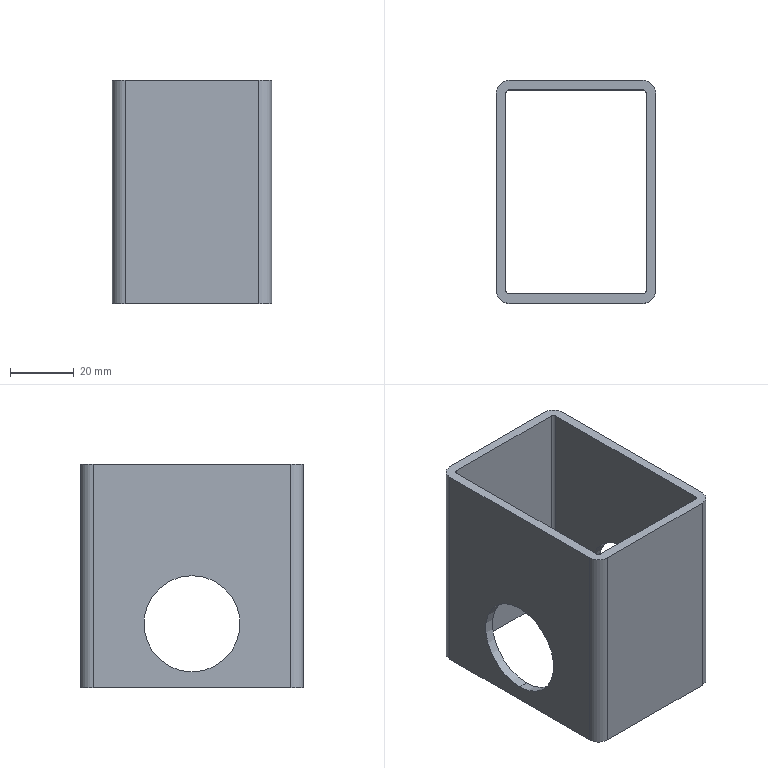Part | SolidWorks | features ExtruThin 1, ICE 1 | 1 solid | 22 faces | box 50 x 70 x 70 mm | volume 42681 mm3 | cylinder 12 | plane 10 | commonest cylinder face diameters 2 x4 8 x4 30.2 x4
STEP:
#1=CARTESIAN_POINT('',(22.,0.,4.9));
#2=VERTEX_POINT('',#1);
#3=CARTESIAN_POINT('',(22.,0.,35.1));
#4=VERTEX_POINT('',#3);
#5=CARTESIAN_POINT('',(22.,0.,20.));
#6=DIRECTION('',(-1.,0.,0.));
#7=DIRECTION('',(0.,0.,1.));
#8=AXIS2_PLACEMENT_3D('',#5,#6,#7);
#9=CIRCLE('',#8,15.1);
#10=EDGE_CURVE('',#2,#4,#9,.T.);
#11=ORIENTED_EDGE('',*,*,#10,.T.);
#12=CARTESIAN_POINT('',(25.,0.,35.1));
#13=VERTEX_POINT('',#12);
#14=CARTESIAN_POINT('',(-25.,0.,35.1));
#15=DIRECTION('',(1.,0.,0.));
#16=VECTOR('',#15,1000.);
#17=LINE('',#14,#16);
#18=EDGE_CURVE('',#4,#13,#17,.T.);
#19=ORIENTED_EDGE('',*,*,#18,.T.);
#20=CARTESIAN_POINT('',(25.,0.,4.9));
#21=VERTEX_POINT('',#20);
#22=CARTESIAN_POINT('',(25.,0.,20.));
#23=DIRECTION('',(1.,0.,0.));
#24=DIRECTION('',(0.,0.,-1.));
#25=AXIS2_PLACEMENT_3D('',#22,#23,#24);
#26=CIRCLE('',#25,15.1);
#27=EDGE_CURVE('',#13,#21,#26,.T.);
#28=ORIENTED_EDGE('',*,*,#27,.T.);
#29=CARTESIAN_POINT('',(-25.,0.,4.9));
#30=DIRECTION('',(1.,0.,0.));
#31=VECTOR('',#30,1000.);
#32=LINE('',#29,#31);
#33=EDGE_CURVE('',#2,#21,#32,.T.);
#34=ORIENTED_EDGE('',*,*,#33,.F.);
#35=EDGE_LOOP('',(#11,#19,#28,#34));
#36=FACE_OUTER_BOUND('',#35,.T.);
#37=CARTESIAN_POINT('',(-25.,0.,20.));
#38=DIRECTION('',(1.,0.,0.));
#39=DIRECTION('',(0.,0.,-1.));
#40=AXIS2_PLACEMENT_3D('',#37,#38,#39);
#41=CYLINDRICAL_SURFACE('',#40,15.1);
#42=ADVANCED_FACE('',(#36),#41,.F.);
#43=CARTESIAN_POINT('',(-25.,0.,35.1));
#44=VERTEX_POINT('',#43);
#45=CARTESIAN_POINT('',(-25.,0.,4.9));
#46=VERTEX_POINT('',#45);
#47=CARTESIAN_POINT('',(-25.,0.,20.));
#48=DIRECTION('',(1.,0.,0.));
#49=DIRECTION('',(0.,0.,-1.));
#50=AXIS2_PLACEMENT_3D('',#47,#48,#49);
#51=CIRCLE('',#50,15.1);
#52=EDGE_CURVE('',#44,#46,#51,.T.);
#53=ORIENTED_EDGE('',*,*,#52,.F.);
#54=CARTESIAN_POINT('',(-22.,0.,35.1));
#55=VERTEX_POINT('',#54);
#56=CARTESIAN_POINT('',(-25.,0.,35.1));
#57=DIRECTION('',(1.,0.,0.));
#58=VECTOR('',#57,1000.);
#59=LINE('',#56,#58);
#60=EDGE_CURVE('',#44,#55,#59,.T.);
#61=ORIENTED_EDGE('',*,*,#60,.T.);
#62=CARTESIAN_POINT('',(-22.,0.,4.9));
#63=VERTEX_POINT('',#62);
#64=CARTESIAN_POINT('',(-22.,0.,20.));
#65=DIRECTION('',(1.,0.,0.));
#66=DIRECTION('',(0.,0.,-1.));
#67=AXIS2_PLACEMENT_3D('',#64,#65,#66);
#68=CIRCLE('',#67,15.1);
#69=EDGE_CURVE('',#55,#63,#68,.T.);
#70=ORIENTED_EDGE('',*,*,#69,.T.);
#71=CARTESIAN_POINT('',(-25.,0.,4.9));
#72=DIRECTION('',(1.,0.,0.));
#73=VECTOR('',#72,1000.);
#74=LINE('',#71,#73);
#75=EDGE_CURVE('',#46,#63,#74,.T.);
#76=ORIENTED_EDGE('',*,*,#75,.F.);
#77=EDGE_LOOP('',(#53,#61,#70,#76));
#78=FACE_OUTER_BOUND('',#77,.T.);
#79=CARTESIAN_POINT('',(-25.,0.,20.));
#80=DIRECTION('',(1.,0.,0.));
#81=DIRECTION('',(0.,0.,-1.));
#82=AXIS2_PLACEMENT_3D('',#79,#80,#81);
#83=CYLINDRICAL_SURFACE('',#82,15.1);
#84=ADVANCED_FACE('',(#78),#83,.F.);
#85=CARTESIAN_POINT('',(-25.,-31.,70.));
#86=VERTEX_POINT('',#85);
#87=CARTESIAN_POINT('',(-21.,-35.,70.));
#88=VERTEX_POINT('',#87);
#89=CARTESIAN_POINT('',(-21.,-31.,70.));
#90=DIRECTION('',(0.,0.,1.));
#91=DIRECTION('',(-1.,0.,0.));
#92=AXIS2_PLACEMENT_3D('',#89,#90,#91);
#93=CIRCLE('',#92,4.);
#94=EDGE_CURVE('',#86,#88,#93,.T.);
#95=ORIENTED_EDGE('',*,*,#94,.T.);
#96=CARTESIAN_POINT('',(21.,-35.,70.));
#97=VERTEX_POINT('',#96);
#98=CARTESIAN_POINT('',(-21.,-35.,70.));
#99=DIRECTION('',(1.,0.,0.));
#100=VECTOR('',#99,1000.);
#101=LINE('',#98,#100);
#102=EDGE_CURVE('',#88,#97,#101,.T.);
#103=ORIENTED_EDGE('',*,*,#102,.T.);
#104=CARTESIAN_POINT('',(25.,-31.,70.));
#105=VERTEX_POINT('',#104);
#106=CARTESIAN_POINT('',(21.,-31.,70.));
#107=DIRECTION('',(0.,0.,1.));
#108=DIRECTION('',(1.,0.,0.));
#109=AXIS2_PLACEMENT_3D('',#106,#107,#108);
#110=CIRCLE('',#109,4.);
#111=EDGE_CURVE('',#97,#105,#110,.T.);
#112=ORIENTED_EDGE('',*,*,#111,.T.);
#113=CARTESIAN_POINT('',(25.,31.,70.));
#114=VERTEX_POINT('',#113);
#115=CARTESIAN_POINT('',(25.,-31.,70.));
#116=DIRECTION('',(0.,1.,0.));
#117=VECTOR('',#116,1000.);
#118=LINE('',#115,#117);
#119=EDGE_CURVE('',#105,#114,#118,.T.);
#120=ORIENTED_EDGE('',*,*,#119,.T.);
#121=CARTESIAN_POINT('',(21.,35.,70.));
#122=VERTEX_POINT('',#121);
#123=CARTESIAN_POINT('',(21.,31.,70.));
#124=DIRECTION('',(0.,0.,1.));
#125=DIRECTION('',(-1.,0.,0.));
#126=AXIS2_PLACEMENT_3D('',#123,#124,#125);
#127=CIRCLE('',#126,4.);
#128=EDGE_CURVE('',#114,#122,#127,.T.);
#129=ORIENTED_EDGE('',*,*,#128,.T.);
#130=CARTESIAN_POINT('',(-21.,35.,70.));
#131=VERTEX_POINT('',#130);
#132=CARTESIAN_POINT('',(-21.,35.,70.));
#133=DIRECTION('',(-1.,0.,0.));
#134=VECTOR('',#133,1000.);
#135=LINE('',#132,#134);
#136=EDGE_CURVE('',#122,#131,#135,.T.);
#137=ORIENTED_EDGE('',*,*,#136,.T.);
#138=CARTESIAN_POINT('',(-25.,31.,70.));
#139=VERTEX_POINT('',#138);
#140=CARTESIAN_POINT('',(-21.,31.,70.));
#141=DIRECTION('',(0.,0.,1.));
#142=DIRECTION('',(-1.,0.,0.));
#143=AXIS2_PLACEMENT_3D('',#140,#141,#142);
#144=CIRCLE('',#143,4.);
#145=EDGE_CURVE('',#131,#139,#144,.T.);
#146=ORIENTED_EDGE('',*,*,#145,.T.);
#147=CARTESIAN_POINT('',(-25.,-31.,70.));
#148=DIRECTION('',(0.,-1.,0.));
#149=VECTOR('',#148,1000.);
#150=LINE('',#147,#149);
#151=EDGE_CURVE('',#139,#86,#150,.T.);
#152=ORIENTED_EDGE('',*,*,#151,.T.);
#153=EDGE_LOOP('',(#95,#103,#112,#120,#129,#137,#146,#152));
#154=FACE_OUTER_BOUND('',#153,.T.);
#155=CARTESIAN_POINT('',(-21.,-32.,70.));
#156=VERTEX_POINT('',#155);
#157=CARTESIAN_POINT('',(21.,-32.,70.));
#158=VERTEX_POINT('',#157);
#159=CARTESIAN_POINT('',(-21.,-32.,70.));
#160=DIRECTION('',(1.,0.,0.));
#161=VECTOR('',#160,1000.);
#162=LINE('',#159,#161);
#163=EDGE_CURVE('',#156,#158,#162,.T.);
#164=ORIENTED_EDGE('',*,*,#163,.F.);
#165=CARTESIAN_POINT('',(-22.,-31.,70.));
#166=VERTEX_POINT('',#165);
#167=CARTESIAN_POINT('',(-21.,-31.,70.));
#168=DIRECTION('',(0.,0.,1.));
#169=DIRECTION('',(-1.,0.,0.));
#170=AXIS2_PLACEMENT_3D('',#167,#168,#169);
#171=CIRCLE('',#170,1.);
#172=EDGE_CURVE('',#166,#156,#171,.T.);
#173=ORIENTED_EDGE('',*,*,#172,.F.);
#174=CARTESIAN_POINT('',(-22.,31.,70.));
#175=VERTEX_POINT('',#174);
#176=CARTESIAN_POINT('',(-22.,-31.,70.));
#177=DIRECTION('',(0.,-1.,0.));
#178=VECTOR('',#177,1000.);
#179=LINE('',#176,#178);
#180=EDGE_CURVE('',#175,#166,#179,.T.);
#181=ORIENTED_EDGE('',*,*,#180,.F.);
#182=CARTESIAN_POINT('',(-21.,32.,70.));
#183=VERTEX_POINT('',#182);
#184=CARTESIAN_POINT('',(-21.,31.,70.));
#185=DIRECTION('',(0.,0.,1.));
#186=DIRECTION('',(-1.,0.,0.));
#187=AXIS2_PLACEMENT_3D('',#184,#185,#186);
#188=CIRCLE('',#187,1.);
#189=EDGE_CURVE('',#183,#175,#188,.T.);
#190=ORIENTED_EDGE('',*,*,#189,.F.);
#191=CARTESIAN_POINT('',(21.,32.,70.));
#192=VERTEX_POINT('',#191);
#193=CARTESIAN_POINT('',(-21.,32.,70.));
#194=DIRECTION('',(-1.,0.,0.));
#195=VECTOR('',#194,1000.);
#196=LINE('',#193,#195);
#197=EDGE_CURVE('',#192,#183,#196,.T.);
#198=ORIENTED_EDGE('',*,*,#197,.F.);
#199=CARTESIAN_POINT('',(22.,31.,70.));
#200=VERTEX_POINT('',#199);
#201=CARTESIAN_POINT('',(21.,31.,70.));
#202=DIRECTION('',(0.,0.,1.));
#203=DIRECTION('',(-1.,0.,0.));
#204=AXIS2_PLACEMENT_3D('',#201,#202,#203);
#205=CIRCLE('',#204,1.);
#206=EDGE_CURVE('',#200,#192,#205,.T.);
#207=ORIENTED_EDGE('',*,*,#206,.F.);
#208=CARTESIAN_POINT('',(22.,-31.,70.));
#209=VERTEX_POINT('',#208);
#210=CARTESIAN_POINT('',(22.,-31.,70.));
#211=DIRECTION('',(0.,1.,0.));
#212=VECTOR('',#211,1000.);
#213=LINE('',#210,#212);
#214=EDGE_CURVE('',#209,#200,#213,.T.);
#215=ORIENTED_EDGE('',*,*,#214,.F.);
#216=CARTESIAN_POINT('',(21.,-31.,70.));
#217=DIRECTION('',(0.,0.,1.));
#218=DIRECTION('',(-1.,0.,0.));
#219=AXIS2_PLACEMENT_3D('',#216,#217,#218);
#220=CIRCLE('',#219,1.);
#221=EDGE_CURVE('',#158,#209,#220,.T.);
#222=ORIENTED_EDGE('',*,*,#221,.F.);
#223=EDGE_LOOP('',(#164,#173,#181,#190,#198,#207,#215,#222));
#224=FACE_BOUND('',#223,.T.);
#225=CARTESIAN_POINT('',(-21.,-31.,70.));
#226=DIRECTION('',(0.,0.,1.));
#227=DIRECTION('',(1.,0.,0.));
#228=AXIS2_PLACEMENT_3D('',#225,#226,#227);
#229=PLANE('',#228);
#230=ADVANCED_FACE('',(#154,#224),#229,.T.);
#231=CARTESIAN_POINT('',(-25.,-31.,0.));
#232=VERTEX_POINT('',#231);
#233=CARTESIAN_POINT('',(-21.,-35.,0.));
#234=VERTEX_POINT('',#233);
#235=CARTESIAN_POINT('',(-21.,-31.,0.));
#236=DIRECTION('',(0.,0.,1.));
#237=DIRECTION('',(-1.,0.,0.));
#238=AXIS2_PLACEMENT_3D('',#235,#236,#237);
#239=CIRCLE('',#238,4.);
#240=EDGE_CURVE('',#232,#234,#239,.T.);
#241=ORIENTED_EDGE('',*,*,#240,.F.);
#242=CARTESIAN_POINT('',(-25.,31.,0.));
#243=VERTEX_POINT('',#242);
#244=CARTESIAN_POINT('',(-25.,-31.,0.));
#245=DIRECTION('',(0.,-1.,0.));
#246=VECTOR('',#245,1000.);
#247=LINE('',#244,#246);
#248=EDGE_CURVE('',#243,#232,#247,.T.);
#249=ORIENTED_EDGE('',*,*,#248,.F.);
#250=CARTESIAN_POINT('',(-21.,35.,0.));
#251=VERTEX_POINT('',#250);
#252=CARTESIAN_POINT('',(-21.,31.,0.));
#253=DIRECTION('',(0.,0.,1.));
#254=DIRECTION('',(-1.,0.,0.));
#255=AXIS2_PLACEMENT_3D('',#252,#253,#254);
#256=CIRCLE('',#255,4.);
#257=EDGE_CURVE('',#251,#243,#256,.T.);
#258=ORIENTED_EDGE('',*,*,#257,.F.);
#259=CARTESIAN_POINT('',(21.,35.,0.));
#260=VERTEX_POINT('',#259);
#261=CARTESIAN_POINT('',(-21.,35.,0.));
#262=DIRECTION('',(-1.,0.,0.));
#263=VECTOR('',#262,1000.);
#264=LINE('',#261,#263);
#265=EDGE_CURVE('',#260,#251,#264,.T.);
#266=ORIENTED_EDGE('',*,*,#265,.F.);
#267=CARTESIAN_POINT('',(25.,31.,0.));
#268=VERTEX_POINT('',#267);
#269=CARTESIAN_POINT('',(21.,31.,0.));
#270=DIRECTION('',(0.,0.,1.));
#271=DIRECTION('',(-1.,0.,0.));
#272=AXIS2_PLACEMENT_3D('',#269,#270,#271);
#273=CIRCLE('',#272,4.);
#274=EDGE_CURVE('',#268,#260,#273,.T.);
#275=ORIENTED_EDGE('',*,*,#274,.F.);
#276=CARTESIAN_POINT('',(25.,-31.,0.));
#277=VERTEX_POINT('',#276);
#278=CARTESIAN_POINT('',(25.,-31.,0.));
#279=DIRECTION('',(0.,1.,0.));
#280=VECTOR('',#279,1000.);
#281=LINE('',#278,#280);
#282=EDGE_CURVE('',#277,#268,#281,.T.);
#283=ORIENTED_EDGE('',*,*,#282,.F.);
#284=CARTESIAN_POINT('',(21.,-35.,0.));
#285=VERTEX_POINT('',#284);
#286=CARTESIAN_POINT('',(21.,-31.,0.));
#287=DIRECTION('',(0.,0.,1.));
#288=DIRECTION('',(1.,0.,0.));
#289=AXIS2_PLACEMENT_3D('',#286,#287,#288);
#290=CIRCLE('',#289,4.);
#291=EDGE_CURVE('',#285,#277,#290,.T.);
#292=ORIENTED_EDGE('',*,*,#291,.F.);
#293=CARTESIAN_POINT('',(-21.,-35.,0.));
#294=DIRECTION('',(1.,0.,0.));
#295=VECTOR('',#294,1000.);
#296=LINE('',#293,#295);
#297=EDGE_CURVE('',#234,#285,#296,.T.);
#298=ORIENTED_EDGE('',*,*,#297,.F.);
#299=EDGE_LOOP('',(#241,#249,#258,#266,#275,#283,#292,#298));
#300=FACE_OUTER_BOUND('',#299,.T.);
#301=CARTESIAN_POINT('',(-22.,-31.,0.));
#302=VERTEX_POINT('',#301);
#303=CARTESIAN_POINT('',(-21.,-32.,0.));
#304=VERTEX_POINT('',#303);
#305=CARTESIAN_POINT('',(-21.,-31.,0.));
#306=DIRECTION('',(0.,0.,1.));
#307=DIRECTION('',(-1.,0.,0.));
#308=AXIS2_PLACEMENT_3D('',#305,#306,#307);
#309=CIRCLE('',#308,1.);
#310=EDGE_CURVE('',#302,#304,#309,.T.);
#311=ORIENTED_EDGE('',*,*,#310,.T.);
#312=CARTESIAN_POINT('',(21.,-32.,0.));
#313=VERTEX_POINT('',#312);
#314=CARTESIAN_POINT('',(-21.,-32.,0.));
#315=DIRECTION('',(1.,0.,0.));
#316=VECTOR('',#315,1000.);
#317=LINE('',#314,#316);
#318=EDGE_CURVE('',#304,#313,#317,.T.);
#319=ORIENTED_EDGE('',*,*,#318,.T.);
#320=CARTESIAN_POINT('',(22.,-31.,0.));
#321=VERTEX_POINT('',#320);
#322=CARTESIAN_POINT('',(21.,-31.,0.));
#323=DIRECTION('',(0.,0.,1.));
#324=DIRECTION('',(-1.,0.,0.));
#325=AXIS2_PLACEMENT_3D('',#322,#323,#324);
#326=CIRCLE('',#325,1.);
#327=EDGE_CURVE('',#313,#321,#326,.T.);
#328=ORIENTED_EDGE('',*,*,#327,.T.);
#329=CARTESIAN_POINT('',(22.,31.,0.));
#330=VERTEX_POINT('',#329);
#331=CARTESIAN_POINT('',(22.,-31.,0.));
#332=DIRECTION('',(0.,1.,0.));
#333=VECTOR('',#332,1000.);
#334=LINE('',#331,#333);
#335=EDGE_CURVE('',#321,#330,#334,.T.);
#336=ORIENTED_EDGE('',*,*,#335,.T.);
#337=CARTESIAN_POINT('',(21.,32.,0.));
#338=VERTEX_POINT('',#337);
#339=CARTESIAN_POINT('',(21.,31.,0.));
#340=DIRECTION('',(0.,0.,1.));
#341=DIRECTION('',(-1.,0.,0.));
#342=AXIS2_PLACEMENT_3D('',#339,#340,#341);
#343=CIRCLE('',#342,1.);
#344=EDGE_CURVE('',#330,#338,#343,.T.);
#345=ORIENTED_EDGE('',*,*,#344,.T.);
#346=CARTESIAN_POINT('',(-21.,32.,0.));
#347=VERTEX_POINT('',#346);
#348=CARTESIAN_POINT('',(-21.,32.,0.));
#349=DIRECTION('',(-1.,0.,0.));
#350=VECTOR('',#349,1000.);
#351=LINE('',#348,#350);
#352=EDGE_CURVE('',#338,#347,#351,.T.);
#353=ORIENTED_EDGE('',*,*,#352,.T.);
#354=CARTESIAN_POINT('',(-22.,31.,0.));
#355=VERTEX_POINT('',#354);
#356=CARTESIAN_POINT('',(-21.,31.,0.));
#357=DIRECTION('',(0.,0.,1.));
#358=DIRECTION('',(-1.,0.,0.));
#359=AXIS2_PLACEMENT_3D('',#356,#357,#358);
#360=CIRCLE('',#359,1.);
#361=EDGE_CURVE('',#347,#355,#360,.T.);
#362=ORIENTED_EDGE('',*,*,#361,.T.);
#363=CARTESIAN_POINT('',(-22.,-31.,0.));
#364=DIRECTION('',(0.,-1.,0.));
#365=VECTOR('',#364,1000.);
#366=LINE('',#363,#365);
#367=EDGE_CURVE('',#355,#302,#366,.T.);
#368=ORIENTED_EDGE('',*,*,#367,.T.);
#369=EDGE_LOOP('',(#311,#319,#328,#336,#345,#353,#362,#368));
#370=FACE_BOUND('',#369,.T.);
#371=CARTESIAN_POINT('',(-21.,-31.,0.));
#372=DIRECTION('',(0.,0.,1.));
#373=DIRECTION('',(1.,0.,0.));
#374=AXIS2_PLACEMENT_3D('',#371,#372,#373);
#375=PLANE('',#374);
#376=ADVANCED_FACE('',(#300,#370),#375,.F.);
#377=ORIENTED_EDGE('',*,*,#240,.T.);
#378=CARTESIAN_POINT('',(-21.,-35.,70.));
#379=DIRECTION('',(0.,0.,-1.));
#380=VECTOR('',#379,1000.);
#381=LINE('',#378,#380);
#382=EDGE_CURVE('',#88,#234,#381,.T.);
#383=ORIENTED_EDGE('',*,*,#382,.F.);
#384=ORIENTED_EDGE('',*,*,#94,.F.);
#385=CARTESIAN_POINT('',(-25.,-31.,70.));
#386=DIRECTION('',(0.,0.,-1.));
#387=VECTOR('',#386,1000.);
#388=LINE('',#385,#387);
#389=EDGE_CURVE('',#86,#232,#388,.T.);
#390=ORIENTED_EDGE('',*,*,#389,.T.);
#391=EDGE_LOOP('',(#377,#383,#384,#390));
#392=FACE_OUTER_BOUND('',#391,.T.);
#393=CARTESIAN_POINT('',(-21.,-31.,70.));
#394=DIRECTION('',(0.,0.,-1.));
#395=DIRECTION('',(-1.,0.,0.));
#396=AXIS2_PLACEMENT_3D('',#393,#394,#395);
#397=CYLINDRICAL_SURFACE('',#396,4.);
#398=ADVANCED_FACE('',(#392),#397,.T.);
#399=ORIENTED_EDGE('',*,*,#297,.T.);
#400=CARTESIAN_POINT('',(21.,-35.,70.));
#401=DIRECTION('',(0.,0.,-1.));
#402=VECTOR('',#401,1000.);
#403=LINE('',#400,#402);
#404=EDGE_CURVE('',#97,#285,#403,.T.);
#405=ORIENTED_EDGE('',*,*,#404,.F.);
#406=ORIENTED_EDGE('',*,*,#102,.F.);
#407=ORIENTED_EDGE('',*,*,#382,.T.);
#408=EDGE_LOOP('',(#399,#405,#406,#407));
#409=FACE_OUTER_BOUND('',#408,.T.);
#410=CARTESIAN_POINT('',(-21.,-35.,70.));
#411=DIRECTION('',(0.,1.,0.));
#412=DIRECTION('',(0.,0.,1.));
#413=AXIS2_PLACEMENT_3D('',#410,#411,#412);
#414=PLANE('',#413);
#415=ADVANCED_FACE('',(#409),#414,.F.);
#416=ORIENTED_EDGE('',*,*,#291,.T.);
#417=CARTESIAN_POINT('',(25.,-31.,70.));
#418=DIRECTION('',(0.,0.,-1.));
#419=VECTOR('',#418,1000.);
#420=LINE('',#417,#419);
#421=EDGE_CURVE('',#105,#277,#420,.T.);
#422=ORIENTED_EDGE('',*,*,#421,.F.);
#423=ORIENTED_EDGE('',*,*,#111,.F.);
#424=ORIENTED_EDGE('',*,*,#404,.T.);
#425=EDGE_LOOP('',(#416,#422,#423,#424));
#426=FACE_OUTER_BOUND('',#425,.T.);
#427=CARTESIAN_POINT('',(21.,-31.,70.));
#428=DIRECTION('',(0.,0.,-1.));
#429=DIRECTION('',(-1.,0.,0.));
#430=AXIS2_PLACEMENT_3D('',#427,#428,#429);
#431=CYLINDRICAL_SURFACE('',#430,4.);
#432=ADVANCED_FACE('',(#426),#431,.T.);
#433=CARTESIAN_POINT('',(25.,0.,20.));
#434=DIRECTION('',(1.,0.,0.));
#435=DIRECTION('',(0.,0.,-1.));
#436=AXIS2_PLACEMENT_3D('',#433,#434,#435);
#437=CIRCLE('',#436,15.1);
#438=EDGE_CURVE('',#21,#13,#437,.T.);
#439=ORIENTED_EDGE('',*,*,#438,.F.);
#440=ORIENTED_EDGE('',*,*,#27,.F.);
#441=EDGE_LOOP('',(#439,#440));
#442=FACE_BOUND('',#441,.T.);
#443=ORIENTED_EDGE('',*,*,#282,.T.);
#444=CARTESIAN_POINT('',(25.,31.,70.));
#445=DIRECTION('',(0.,0.,-1.));
#446=VECTOR('',#445,1000.);
#447=LINE('',#444,#446);
#448=EDGE_CURVE('',#114,#268,#447,.T.);
#449=ORIENTED_EDGE('',*,*,#448,.F.);
#450=ORIENTED_EDGE('',*,*,#119,.F.);
#451=ORIENTED_EDGE('',*,*,#421,.T.);
#452=EDGE_LOOP('',(#443,#449,#450,#451));
#453=FACE_OUTER_BOUND('',#452,.T.);
#454=CARTESIAN_POINT('',(25.,-31.,70.));
#455=DIRECTION('',(-1.,0.,0.));
#456=DIRECTION('',(0.,0.,1.));
#457=AXIS2_PLACEMENT_3D('',#454,#455,#456);
#458=PLANE('',#457);
#459=ADVANCED_FACE('',(#442,#453),#458,.F.);
#460=ORIENTED_EDGE('',*,*,#274,.T.);
#461=CARTESIAN_POINT('',(21.,35.,70.));
#462=DIRECTION('',(0.,0.,-1.));
#463=VECTOR('',#462,1000.);
#464=LINE('',#461,#463);
#465=EDGE_CURVE('',#122,#260,#464,.T.);
#466=ORIENTED_EDGE('',*,*,#465,.F.);
#467=ORIENTED_EDGE('',*,*,#128,.F.);
#468=ORIENTED_EDGE('',*,*,#448,.T.);
#469=EDGE_LOOP('',(#460,#466,#467,#468));
#470=FACE_OUTER_BOUND('',#469,.T.);
#471=CARTESIAN_POINT('',(21.,31.,70.));
#472=DIRECTION('',(0.,0.,-1.));
#473=DIRECTION('',(-1.,0.,0.));
#474=AXIS2_PLACEMENT_3D('',#471,#472,#473);
#475=CYLINDRICAL_SURFACE('',#474,4.);
#476=ADVANCED_FACE('',(#470),#475,.T.);
#477=ORIENTED_EDGE('',*,*,#265,.T.);
#478=CARTESIAN_POINT('',(-21.,35.,70.));
#479=DIRECTION('',(0.,0.,-1.));
#480=VECTOR('',#479,1000.);
#481=LINE('',#478,#480);
#482=EDGE_CURVE('',#131,#251,#481,.T.);
#483=ORIENTED_EDGE('',*,*,#482,.F.);
#484=ORIENTED_EDGE('',*,*,#136,.F.);
#485=ORIENTED_EDGE('',*,*,#465,.T.);
#486=EDGE_LOOP('',(#477,#483,#484,#485));
#487=FACE_OUTER_BOUND('',#486,.T.);
#488=CARTESIAN_POINT('',(-21.,35.,70.));
#489=DIRECTION('',(0.,-1.,0.));
#490=DIRECTION('',(0.,0.,-1.));
#491=AXIS2_PLACEMENT_3D('',#488,#489,#490);
#492=PLANE('',#491);
#493=ADVANCED_FACE('',(#487),#492,.F.);
#494=ORIENTED_EDGE('',*,*,#257,.T.);
#495=CARTESIAN_POINT('',(-25.,31.,70.));
#496=DIRECTION('',(0.,0.,-1.));
#497=VECTOR('',#496,1000.);
#498=LINE('',#495,#497);
#499=EDGE_CURVE('',#139,#243,#498,.T.);
#500=ORIENTED_EDGE('',*,*,#499,.F.);
#501=ORIENTED_EDGE('',*,*,#145,.F.);
#502=ORIENTED_EDGE('',*,*,#482,.T.);
#503=EDGE_LOOP('',(#494,#500,#501,#502));
#504=FACE_OUTER_BOUND('',#503,.T.);
#505=CARTESIAN_POINT('',(-21.,31.,70.));
#506=DIRECTION('',(0.,0.,-1.));
#507=DIRECTION('',(-1.,0.,0.));
#508=AXIS2_PLACEMENT_3D('',#505,#506,#507);
#509=CYLINDRICAL_SURFACE('',#508,4.);
#510=ADVANCED_FACE('',(#504),#509,.T.);
#511=CARTESIAN_POINT('',(-25.,0.,20.));
#512=DIRECTION('',(1.,0.,0.));
#513=DIRECTION('',(0.,0.,-1.));
#514=AXIS2_PLACEMENT_3D('',#511,#512,#513);
#515=CIRCLE('',#514,15.1);
#516=EDGE_CURVE('',#46,#44,#515,.T.);
#517=ORIENTED_EDGE('',*,*,#516,.T.);
#518=ORIENTED_EDGE('',*,*,#52,.T.);
#519=EDGE_LOOP('',(#517,#518));
#520=FACE_BOUND('',#519,.T.);
#521=ORIENTED_EDGE('',*,*,#248,.T.);
#522=ORIENTED_EDGE('',*,*,#389,.F.);
#523=ORIENTED_EDGE('',*,*,#151,.F.);
#524=ORIENTED_EDGE('',*,*,#499,.T.);
#525=EDGE_LOOP('',(#521,#522,#523,#524));
#526=FACE_OUTER_BOUND('',#525,.T.);
#527=CARTESIAN_POINT('',(-25.,-31.,70.));
#528=DIRECTION('',(1.,0.,0.));
#529=DIRECTION('',(0.,0.,-1.));
#530=AXIS2_PLACEMENT_3D('',#527,#528,#529);
#531=PLANE('',#530);
#532=ADVANCED_FACE('',(#520,#526),#531,.F.);
#533=ORIENTED_EDGE('',*,*,#310,.F.);
#534=CARTESIAN_POINT('',(-22.,-31.,70.));
#535=DIRECTION('',(0.,0.,-1.));
#536=VECTOR('',#535,1000.);
#537=LINE('',#534,#536);
#538=EDGE_CURVE('',#166,#302,#537,.T.);
#539=ORIENTED_EDGE('',*,*,#538,.F.);
#540=ORIENTED_EDGE('',*,*,#172,.T.);
#541=CARTESIAN_POINT('',(-21.,-32.,70.));
#542=DIRECTION('',(0.,0.,-1.));
#543=VECTOR('',#542,1000.);
#544=LINE('',#541,#543);
#545=EDGE_CURVE('',#156,#304,#544,.T.);
#546=ORIENTED_EDGE('',*,*,#545,.T.);
#547=EDGE_LOOP('',(#533,#539,#540,#546));
#548=FACE_OUTER_BOUND('',#547,.T.);
#549=CARTESIAN_POINT('',(-21.,-31.,70.));
#550=DIRECTION('',(0.,0.,-1.));
#551=DIRECTION('',(-1.,0.,0.));
#552=AXIS2_PLACEMENT_3D('',#549,#550,#551);
#553=CYLINDRICAL_SURFACE('',#552,1.);
#554=ADVANCED_FACE('',(#548),#553,.F.);
#555=ORIENTED_EDGE('',*,*,#318,.F.);
#556=ORIENTED_EDGE('',*,*,#545,.F.);
#557=ORIENTED_EDGE('',*,*,#163,.T.);
#558=CARTESIAN_POINT('',(21.,-32.,70.));
#559=DIRECTION('',(0.,0.,-1.));
#560=VECTOR('',#559,1000.);
#561=LINE('',#558,#560);
#562=EDGE_CURVE('',#158,#313,#561,.T.);
#563=ORIENTED_EDGE('',*,*,#562,.T.);
#564=EDGE_LOOP('',(#555,#556,#557,#563));
#565=FACE_OUTER_BOUND('',#564,.T.);
#566=CARTESIAN_POINT('',(-21.,-32.,70.));
#567=DIRECTION('',(0.,1.,0.));
#568=DIRECTION('',(0.,0.,1.));
#569=AXIS2_PLACEMENT_3D('',#566,#567,#568);
#570=PLANE('',#569);
#571=ADVANCED_FACE('',(#565),#570,.T.);
#572=ORIENTED_EDGE('',*,*,#327,.F.);
#573=ORIENTED_EDGE('',*,*,#562,.F.);
#574=ORIENTED_EDGE('',*,*,#221,.T.);
#575=CARTESIAN_POINT('',(22.,-31.,70.));
#576=DIRECTION('',(0.,0.,-1.));
#577=VECTOR('',#576,1000.);
#578=LINE('',#575,#577);
#579=EDGE_CURVE('',#209,#321,#578,.T.);
#580=ORIENTED_EDGE('',*,*,#579,.T.);
#581=EDGE_LOOP('',(#572,#573,#574,#580));
#582=FACE_OUTER_BOUND('',#581,.T.);
#583=CARTESIAN_POINT('',(21.,-31.,70.));
#584=DIRECTION('',(0.,0.,-1.));
#585=DIRECTION('',(-1.,0.,0.));
#586=AXIS2_PLACEMENT_3D('',#583,#584,#585);
#587=CYLINDRICAL_SURFACE('',#586,1.);
#588=ADVANCED_FACE('',(#582),#587,.F.);
#589=ORIENTED_EDGE('',*,*,#10,.F.);
#590=CARTESIAN_POINT('',(22.,0.,20.));
#591=DIRECTION('',(-1.,0.,0.));
#592=DIRECTION('',(0.,0.,1.));
#593=AXIS2_PLACEMENT_3D('',#590,#591,#592);
#594=CIRCLE('',#593,15.1);
#595=EDGE_CURVE('',#4,#2,#594,.T.);
#596=ORIENTED_EDGE('',*,*,#595,.F.);
#597=EDGE_LOOP('',(#589,#596));
#598=FACE_BOUND('',#597,.T.);
#599=ORIENTED_EDGE('',*,*,#335,.F.);
#600=ORIENTED_EDGE('',*,*,#579,.F.);
#601=ORIENTED_EDGE('',*,*,#214,.T.);
#602=CARTESIAN_POINT('',(22.,31.,70.));
#603=DIRECTION('',(0.,0.,-1.));
#604=VECTOR('',#603,1000.);
#605=LINE('',#602,#604);
#606=EDGE_CURVE('',#200,#330,#605,.T.);
#607=ORIENTED_EDGE('',*,*,#606,.T.);
#608=EDGE_LOOP('',(#599,#600,#601,#607));
#609=FACE_OUTER_BOUND('',#608,.T.);
#610=CARTESIAN_POINT('',(22.,-31.,70.));
#611=DIRECTION('',(-1.,0.,0.));
#612=DIRECTION('',(0.,0.,1.));
#613=AXIS2_PLACEMENT_3D('',#610,#611,#612);
#614=PLANE('',#613);
#615=ADVANCED_FACE('',(#598,#609),#614,.T.);
#616=ORIENTED_EDGE('',*,*,#344,.F.);
#617=ORIENTED_EDGE('',*,*,#606,.F.);
#618=ORIENTED_EDGE('',*,*,#206,.T.);
#619=CARTESIAN_POINT('',(21.,32.,70.));
#620=DIRECTION('',(0.,0.,-1.));
#621=VECTOR('',#620,1000.);
#622=LINE('',#619,#621);
#623=EDGE_CURVE('',#192,#338,#622,.T.);
#624=ORIENTED_EDGE('',*,*,#623,.T.);
#625=EDGE_LOOP('',(#616,#617,#618,#624));
#626=FACE_OUTER_BOUND('',#625,.T.);
#627=CARTESIAN_POINT('',(21.,31.,70.));
#628=DIRECTION('',(0.,0.,-1.));
#629=DIRECTION('',(-1.,0.,0.));
#630=AXIS2_PLACEMENT_3D('',#627,#628,#629);
#631=CYLINDRICAL_SURFACE('',#630,1.);
#632=ADVANCED_FACE('',(#626),#631,.F.);
#633=ORIENTED_EDGE('',*,*,#352,.F.);
#634=ORIENTED_EDGE('',*,*,#623,.F.);
#635=ORIENTED_EDGE('',*,*,#197,.T.);
#636=CARTESIAN_POINT('',(-21.,32.,70.));
#637=DIRECTION('',(0.,0.,-1.));
#638=VECTOR('',#637,1000.);
#639=LINE('',#636,#638);
#640=EDGE_CURVE('',#183,#347,#639,.T.);
#641=ORIENTED_EDGE('',*,*,#640,.T.);
#642=EDGE_LOOP('',(#633,#634,#635,#641));
#643=FACE_OUTER_BOUND('',#642,.T.);
#644=CARTESIAN_POINT('',(-21.,32.,70.));
#645=DIRECTION('',(0.,-1.,0.));
#646=DIRECTION('',(0.,0.,-1.));
#647=AXIS2_PLACEMENT_3D('',#644,#645,#646);
#648=PLANE('',#647);
#649=ADVANCED_FACE('',(#643),#648,.T.);
#650=ORIENTED_EDGE('',*,*,#361,.F.);
#651=ORIENTED_EDGE('',*,*,#640,.F.);
#652=ORIENTED_EDGE('',*,*,#189,.T.);
#653=CARTESIAN_POINT('',(-22.,31.,70.));
#654=DIRECTION('',(0.,0.,-1.));
#655=VECTOR('',#654,1000.);
#656=LINE('',#653,#655);
#657=EDGE_CURVE('',#175,#355,#656,.T.);
#658=ORIENTED_EDGE('',*,*,#657,.T.);
#659=EDGE_LOOP('',(#650,#651,#652,#658));
#660=FACE_OUTER_BOUND('',#659,.T.);
#661=CARTESIAN_POINT('',(-21.,31.,70.));
#662=DIRECTION('',(0.,0.,-1.));
#663=DIRECTION('',(-1.,0.,0.));
#664=AXIS2_PLACEMENT_3D('',#661,#662,#663);
#665=CYLINDRICAL_SURFACE('',#664,1.);
#666=ADVANCED_FACE('',(#660),#665,.F.);
#667=CARTESIAN_POINT('',(-22.,0.,20.));
#668=DIRECTION('',(1.,0.,0.));
#669=DIRECTION('',(0.,0.,-1.));
#670=AXIS2_PLACEMENT_3D('',#667,#668,#669);
#671=CIRCLE('',#670,15.1);
#672=EDGE_CURVE('',#63,#55,#671,.T.);
#673=ORIENTED_EDGE('',*,*,#672,.F.);
#674=ORIENTED_EDGE('',*,*,#69,.F.);
#675=EDGE_LOOP('',(#673,#674));
#676=FACE_BOUND('',#675,.T.);
#677=ORIENTED_EDGE('',*,*,#367,.F.);
#678=ORIENTED_EDGE('',*,*,#657,.F.);
#679=ORIENTED_EDGE('',*,*,#180,.T.);
#680=ORIENTED_EDGE('',*,*,#538,.T.);
#681=EDGE_LOOP('',(#677,#678,#679,#680));
#682=FACE_OUTER_BOUND('',#681,.T.);
#683=CARTESIAN_POINT('',(-22.,-31.,70.));
#684=DIRECTION('',(1.,0.,0.));
#685=DIRECTION('',(0.,0.,-1.));
#686=AXIS2_PLACEMENT_3D('',#683,#684,#685);
#687=PLANE('',#686);
#688=ADVANCED_FACE('',(#676,#682),#687,.T.);
#689=ORIENTED_EDGE('',*,*,#60,.F.);
#690=ORIENTED_EDGE('',*,*,#516,.F.);
#691=ORIENTED_EDGE('',*,*,#75,.T.);
#692=ORIENTED_EDGE('',*,*,#672,.T.);
#693=EDGE_LOOP('',(#689,#690,#691,#692));
#694=FACE_OUTER_BOUND('',#693,.T.);
#695=CARTESIAN_POINT('',(-25.,0.,20.));
#696=DIRECTION('',(1.,0.,0.));
#697=DIRECTION('',(0.,0.,-1.));
#698=AXIS2_PLACEMENT_3D('',#695,#696,#697);
#699=CYLINDRICAL_SURFACE('',#698,15.1);
#700=ADVANCED_FACE('',(#694),#699,.F.);
#701=ORIENTED_EDGE('',*,*,#18,.F.);
#702=ORIENTED_EDGE('',*,*,#595,.T.);
#703=ORIENTED_EDGE('',*,*,#33,.T.);
#704=ORIENTED_EDGE('',*,*,#438,.T.);
#705=EDGE_LOOP('',(#701,#702,#703,#704));
#706=FACE_OUTER_BOUND('',#705,.T.);
#707=CARTESIAN_POINT('',(-25.,0.,20.));
#708=DIRECTION('',(1.,0.,0.));
#709=DIRECTION('',(0.,0.,-1.));
#710=AXIS2_PLACEMENT_3D('',#707,#708,#709);
#711=CYLINDRICAL_SURFACE('',#710,15.1);
#712=ADVANCED_FACE('',(#706),#711,.F.);
#713=CLOSED_SHELL('',(#42,#84,#230,#376,#398,#415,#432,#459,#476,#493,#510,#532,#554,#571,#588,#615,#632,#649,#666,#688,#700,#712));
#714=MANIFOLD_SOLID_BREP('',#713);
#715=CARTESIAN_POINT('',(0.,0.,0.));
#716=DIRECTION('',(0.,0.,1.));
#717=DIRECTION('',(1.,0.,0.));
#718=AXIS2_PLACEMENT_3D('',#715,#716,#717);
#719=(LENGTH_UNIT()NAMED_UNIT(*)SI_UNIT(.MILLI.,.METRE.));
#720=UNCERTAINTY_MEASURE_WITH_UNIT(LENGTH_MEASURE(0.00001),#719,'','');
#721=(NAMED_UNIT(*)PLANE_ANGLE_UNIT()SI_UNIT($,.RADIAN.));
#722=(NAMED_UNIT(*)SI_UNIT($,.STERADIAN.)SOLID_ANGLE_UNIT());
#723=(GEOMETRIC_REPRESENTATION_CONTEXT(3)GLOBAL_UNCERTAINTY_ASSIGNED_CONTEXT((#720))GLOBAL_UNIT_ASSIGNED_CONTEXT((#719,#721,#722))REPRESENTATION_CONTEXT('',''));
#724=ADVANCED_BREP_SHAPE_REPRESENTATION('',(#714,#718),#723);